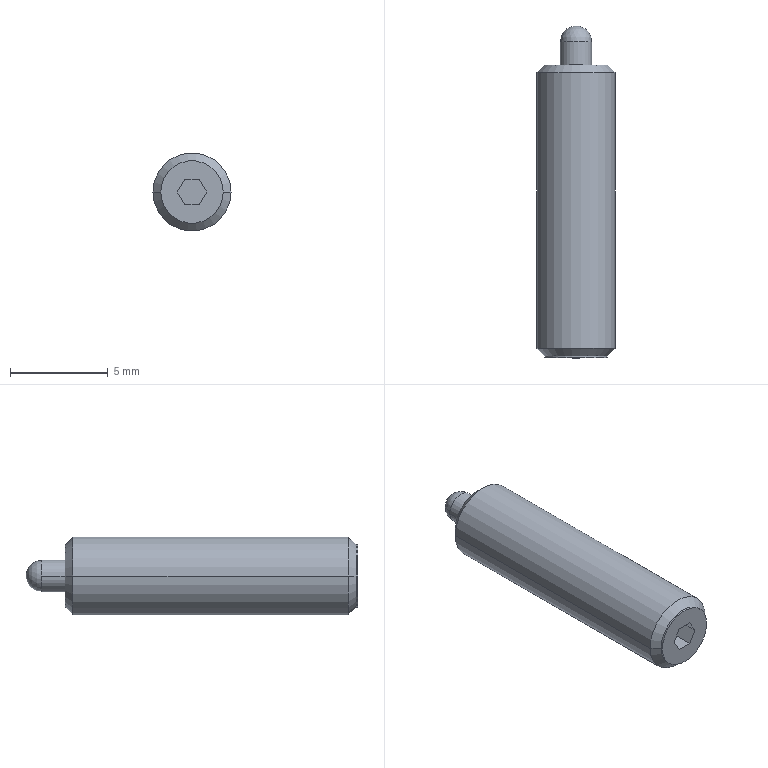Part | NX | 1 solid | 20 faces | box 4 x 17 x 4 mm | volume 187.749 mm3 | plane 9 | cylinder 6 | cone 4 | sphere 1 | commonest cylinder face diameters 1.6 x2 3.2 x2 4 x2
STEP:
#1=CARTESIAN_POINT('',(0.8,16.2,0.));
#2=VERTEX_POINT('',#1);
#3=CARTESIAN_POINT('',(-0.8,16.2,0.));
#4=VERTEX_POINT('',#3);
#5=CARTESIAN_POINT('',(0.,16.2,0.));
#6=DIRECTION('',(0.,1.,0.));
#7=DIRECTION('',(1.,0.,0.));
#8=AXIS2_PLACEMENT_3D('',#5,#6,#7);
#9=CIRCLE('',#8,0.8);
#10=EDGE_CURVE('',#2,#4,#9,.T.);
#11=ORIENTED_EDGE('',*,*,#10,.T.);
#12=CARTESIAN_POINT('',(0.,16.2,0.));
#13=DIRECTION('',(0.,1.,0.));
#14=DIRECTION('',(1.,0.,0.));
#15=AXIS2_PLACEMENT_3D('',#12,#13,#14);
#16=CIRCLE('',#15,0.8);
#17=EDGE_CURVE('',#4,#2,#16,.T.);
#18=ORIENTED_EDGE('',*,*,#17,.T.);
#19=EDGE_LOOP('',(#11,#18));
#20=FACE_BOUND('',#19,.T.);
#21=CARTESIAN_POINT('',(0.,16.2,0.));
#22=DIRECTION('',(0.,1.,0.));
#23=DIRECTION('',(1.,0.,0.));
#24=AXIS2_PLACEMENT_3D('',#21,#22,#23);
#25=SPHERICAL_SURFACE('',#24,0.8);
#26=ADVANCED_FACE('',(#20),#25,.T.);
#27=CARTESIAN_POINT('',(-0.7506,0.,0.));
#28=VERTEX_POINT('',#27);
#29=CARTESIAN_POINT('',(-0.3753,0.,-0.65));
#30=VERTEX_POINT('',#29);
#31=CARTESIAN_POINT('',(-0.7506,0.,0.));
#32=DIRECTION('',(0.5,0.,-0.866));
#33=VECTOR('',#32,1000.);
#34=LINE('',#31,#33);
#35=EDGE_CURVE('',#28,#30,#34,.T.);
#36=ORIENTED_EDGE('',*,*,#35,.T.);
#37=CARTESIAN_POINT('',(-0.3753,1.3,-0.65));
#38=VERTEX_POINT('',#37);
#39=CARTESIAN_POINT('',(-0.3753,1.3,-0.65));
#40=DIRECTION('',(0.,-1.,0.));
#41=VECTOR('',#40,1000.);
#42=LINE('',#39,#41);
#43=EDGE_CURVE('',#38,#30,#42,.T.);
#44=ORIENTED_EDGE('',*,*,#43,.F.);
#45=CARTESIAN_POINT('',(-0.7506,1.3,0.));
#46=VERTEX_POINT('',#45);
#47=CARTESIAN_POINT('',(-0.3753,1.3,-0.65));
#48=DIRECTION('',(-0.5,0.,0.866));
#49=VECTOR('',#48,1000.);
#50=LINE('',#47,#49);
#51=EDGE_CURVE('',#38,#46,#50,.T.);
#52=ORIENTED_EDGE('',*,*,#51,.T.);
#53=CARTESIAN_POINT('',(-0.7506,1.3,0.));
#54=DIRECTION('',(0.,-1.,0.));
#55=VECTOR('',#54,1000.);
#56=LINE('',#53,#55);
#57=EDGE_CURVE('',#46,#28,#56,.T.);
#58=ORIENTED_EDGE('',*,*,#57,.T.);
#59=EDGE_LOOP('',(#36,#44,#52,#58));
#60=FACE_BOUND('',#59,.T.);
#61=CARTESIAN_POINT('',(-0.7506,0.,0.));
#62=DIRECTION('',(-0.866,0.,-0.5));
#63=DIRECTION('',(-0.5,0.,0.866));
#64=AXIS2_PLACEMENT_3D('',#61,#62,#63);
#65=PLANE('',#64);
#66=ADVANCED_FACE('',(#60),#65,.F.);
#67=ORIENTED_EDGE('',*,*,#17,.F.);
#68=CARTESIAN_POINT('',(-0.8,15.,0.));
#69=VERTEX_POINT('',#68);
#70=CARTESIAN_POINT('',(-0.8,17.85,0.));
#71=DIRECTION('',(0.,-1.,0.));
#72=VECTOR('',#71,1000.);
#73=LINE('',#70,#72);
#74=EDGE_CURVE('',#69,#4,#73,.F.);
#75=ORIENTED_EDGE('',*,*,#74,.F.);
#76=CARTESIAN_POINT('',(0.8,15.,0.));
#77=VERTEX_POINT('',#76);
#78=CARTESIAN_POINT('',(0.,15.,0.));
#79=DIRECTION('',(0.,1.,0.));
#80=DIRECTION('',(1.,0.,0.));
#81=AXIS2_PLACEMENT_3D('',#78,#79,#80);
#82=CIRCLE('',#81,0.8);
#83=EDGE_CURVE('',#69,#77,#82,.T.);
#84=ORIENTED_EDGE('',*,*,#83,.T.);
#85=CARTESIAN_POINT('',(0.8,17.85,0.));
#86=DIRECTION('',(0.,-1.,0.));
#87=VECTOR('',#86,1000.);
#88=LINE('',#85,#87);
#89=EDGE_CURVE('',#77,#2,#88,.F.);
#90=ORIENTED_EDGE('',*,*,#89,.T.);
#91=EDGE_LOOP('',(#67,#75,#84,#90));
#92=FACE_BOUND('',#91,.T.);
#93=CARTESIAN_POINT('',(0.,17.85,0.));
#94=DIRECTION('',(0.,-1.,0.));
#95=DIRECTION('',(-1.,0.,0.));
#96=AXIS2_PLACEMENT_3D('',#93,#94,#95);
#97=CYLINDRICAL_SURFACE('',#96,0.8);
#98=ADVANCED_FACE('',(#92),#97,.T.);
#99=CARTESIAN_POINT('',(0.3753,0.,-0.65));
#100=VERTEX_POINT('',#99);
#101=CARTESIAN_POINT('',(0.3753,0.,-0.65));
#102=DIRECTION('',(-1.,0.,0.));
#103=VECTOR('',#102,1000.);
#104=LINE('',#101,#103);
#105=EDGE_CURVE('',#100,#30,#104,.T.);
#106=ORIENTED_EDGE('',*,*,#105,.F.);
#107=CARTESIAN_POINT('',(0.3753,1.3,-0.65));
#108=VERTEX_POINT('',#107);
#109=CARTESIAN_POINT('',(0.3753,1.3,-0.65));
#110=DIRECTION('',(0.,-1.,0.));
#111=VECTOR('',#110,1000.);
#112=LINE('',#109,#111);
#113=EDGE_CURVE('',#108,#100,#112,.T.);
#114=ORIENTED_EDGE('',*,*,#113,.F.);
#115=CARTESIAN_POINT('',(0.3753,1.3,-0.65));
#116=DIRECTION('',(-1.,0.,0.));
#117=VECTOR('',#116,1000.);
#118=LINE('',#115,#117);
#119=EDGE_CURVE('',#108,#38,#118,.T.);
#120=ORIENTED_EDGE('',*,*,#119,.T.);
#121=ORIENTED_EDGE('',*,*,#43,.T.);
#122=EDGE_LOOP('',(#106,#114,#120,#121));
#123=FACE_BOUND('',#122,.T.);
#124=CARTESIAN_POINT('',(-0.3753,0.,-0.65));
#125=DIRECTION('',(0.,0.,-1.));
#126=DIRECTION('',(0.,-1.,0.));
#127=AXIS2_PLACEMENT_3D('',#124,#125,#126);
#128=PLANE('',#127);
#129=ADVANCED_FACE('',(#123),#128,.F.);
#130=CARTESIAN_POINT('',(-1.6,15.,0.));
#131=VERTEX_POINT('',#130);
#132=CARTESIAN_POINT('',(1.6,15.,0.));
#133=VERTEX_POINT('',#132);
#134=CARTESIAN_POINT('',(0.,15.,0.));
#135=DIRECTION('',(0.,-1.,0.));
#136=DIRECTION('',(-1.,0.,0.));
#137=AXIS2_PLACEMENT_3D('',#134,#135,#136);
#138=CIRCLE('',#137,1.6);
#139=EDGE_CURVE('',#131,#133,#138,.T.);
#140=ORIENTED_EDGE('',*,*,#139,.F.);
#141=CARTESIAN_POINT('',(0.,15.,0.));
#142=DIRECTION('',(0.,-1.,0.));
#143=DIRECTION('',(-1.,0.,0.));
#144=AXIS2_PLACEMENT_3D('',#141,#142,#143);
#145=CIRCLE('',#144,1.6);
#146=EDGE_CURVE('',#133,#131,#145,.T.);
#147=ORIENTED_EDGE('',*,*,#146,.F.);
#148=EDGE_LOOP('',(#140,#147));
#149=FACE_BOUND('',#148,.T.);
#150=CARTESIAN_POINT('',(0.,15.,0.));
#151=DIRECTION('',(0.,1.,0.));
#152=DIRECTION('',(1.,0.,0.));
#153=AXIS2_PLACEMENT_3D('',#150,#151,#152);
#154=CIRCLE('',#153,0.8);
#155=EDGE_CURVE('',#77,#69,#154,.T.);
#156=ORIENTED_EDGE('',*,*,#155,.F.);
#157=ORIENTED_EDGE('',*,*,#83,.F.);
#158=EDGE_LOOP('',(#156,#157));
#159=FACE_BOUND('',#158,.T.);
#160=CARTESIAN_POINT('',(0.,15.,0.));
#161=DIRECTION('',(0.,-1.,0.));
#162=DIRECTION('',(0.,0.,-1.));
#163=AXIS2_PLACEMENT_3D('',#160,#161,#162);
#164=PLANE('',#163);
#165=ADVANCED_FACE('',(#149,#159),#164,.F.);
#166=ORIENTED_EDGE('',*,*,#139,.T.);
#167=CARTESIAN_POINT('',(2.,14.6,0.));
#168=VERTEX_POINT('',#167);
#169=CARTESIAN_POINT('',(1.8,14.8,0.));
#170=DIRECTION('',(0.7071,-0.7071,0.));
#171=VECTOR('',#170,1000.);
#172=LINE('',#169,#171);
#173=EDGE_CURVE('',#168,#133,#172,.F.);
#174=ORIENTED_EDGE('',*,*,#173,.F.);
#175=CARTESIAN_POINT('',(-2.,14.6,0.));
#176=VERTEX_POINT('',#175);
#177=CARTESIAN_POINT('',(0.,14.6,0.));
#178=DIRECTION('',(0.,-1.,0.));
#179=DIRECTION('',(-1.,0.,0.));
#180=AXIS2_PLACEMENT_3D('',#177,#178,#179);
#181=CIRCLE('',#180,2.);
#182=EDGE_CURVE('',#176,#168,#181,.T.);
#183=ORIENTED_EDGE('',*,*,#182,.F.);
#184=CARTESIAN_POINT('',(-1.8,14.8,0.));
#185=DIRECTION('',(-0.7071,-0.7071,0.));
#186=VECTOR('',#185,1000.);
#187=LINE('',#184,#186);
#188=EDGE_CURVE('',#176,#131,#187,.F.);
#189=ORIENTED_EDGE('',*,*,#188,.T.);
#190=EDGE_LOOP('',(#166,#174,#183,#189));
#191=FACE_BOUND('',#190,.T.);
#192=CARTESIAN_POINT('',(0.,14.8,0.));
#193=DIRECTION('',(0.,-1.,0.));
#194=DIRECTION('',(-1.,0.,0.));
#195=AXIS2_PLACEMENT_3D('',#192,#193,#194);
#196=CONICAL_SURFACE('',#195,1.8,0.7854);
#197=ADVANCED_FACE('',(#191),#196,.T.);
#198=CARTESIAN_POINT('',(0.3753,1.3,0.65));
#199=VERTEX_POINT('',#198);
#200=CARTESIAN_POINT('',(0.7506,1.3,0.));
#201=VERTEX_POINT('',#200);
#202=CARTESIAN_POINT('',(0.3753,1.3,0.65));
#203=DIRECTION('',(0.5,0.,-0.866));
#204=VECTOR('',#203,1000.);
#205=LINE('',#202,#204);
#206=EDGE_CURVE('',#199,#201,#205,.T.);
#207=ORIENTED_EDGE('',*,*,#206,.F.);
#208=CARTESIAN_POINT('',(-0.3753,1.3,0.65));
#209=VERTEX_POINT('',#208);
#210=CARTESIAN_POINT('',(-0.3753,1.3,0.65));
#211=DIRECTION('',(1.,0.,0.));
#212=VECTOR('',#211,1000.);
#213=LINE('',#210,#212);
#214=EDGE_CURVE('',#209,#199,#213,.T.);
#215=ORIENTED_EDGE('',*,*,#214,.F.);
#216=CARTESIAN_POINT('',(-0.7506,1.3,0.));
#217=DIRECTION('',(0.5,0.,0.866));
#218=VECTOR('',#217,1000.);
#219=LINE('',#216,#218);
#220=EDGE_CURVE('',#46,#209,#219,.T.);
#221=ORIENTED_EDGE('',*,*,#220,.F.);
#222=ORIENTED_EDGE('',*,*,#51,.F.);
#223=ORIENTED_EDGE('',*,*,#119,.F.);
#224=CARTESIAN_POINT('',(0.7506,1.3,0.));
#225=DIRECTION('',(-0.5,0.,-0.866));
#226=VECTOR('',#225,1000.);
#227=LINE('',#224,#226);
#228=EDGE_CURVE('',#201,#108,#227,.T.);
#229=ORIENTED_EDGE('',*,*,#228,.F.);
#230=EDGE_LOOP('',(#207,#215,#221,#222,#223,#229));
#231=FACE_BOUND('',#230,.T.);
#232=CARTESIAN_POINT('',(0.,1.3,0.));
#233=DIRECTION('',(0.,-1.,0.));
#234=DIRECTION('',(0.,0.,-1.));
#235=AXIS2_PLACEMENT_3D('',#232,#233,#234);
#236=PLANE('',#235);
#237=ADVANCED_FACE('',(#231),#236,.T.);
#238=ORIENTED_EDGE('',*,*,#182,.T.);
#239=CARTESIAN_POINT('',(2.,0.5,0.));
#240=VERTEX_POINT('',#239);
#241=CARTESIAN_POINT('',(2.,17.85,0.));
#242=DIRECTION('',(0.,-1.,0.));
#243=VECTOR('',#242,1000.);
#244=LINE('',#241,#243);
#245=EDGE_CURVE('',#168,#240,#244,.T.);
#246=ORIENTED_EDGE('',*,*,#245,.T.);
#247=CARTESIAN_POINT('',(-2.,0.5,0.));
#248=VERTEX_POINT('',#247);
#249=CARTESIAN_POINT('',(0.,0.5,0.));
#250=DIRECTION('',(0.,1.,0.));
#251=DIRECTION('',(1.,0.,0.));
#252=AXIS2_PLACEMENT_3D('',#249,#250,#251);
#253=CIRCLE('',#252,2.);
#254=EDGE_CURVE('',#240,#248,#253,.T.);
#255=ORIENTED_EDGE('',*,*,#254,.T.);
#256=CARTESIAN_POINT('',(-2.,17.85,0.));
#257=DIRECTION('',(0.,-1.,0.));
#258=VECTOR('',#257,1000.);
#259=LINE('',#256,#258);
#260=EDGE_CURVE('',#176,#248,#259,.T.);
#261=ORIENTED_EDGE('',*,*,#260,.F.);
#262=EDGE_LOOP('',(#238,#246,#255,#261));
#263=FACE_BOUND('',#262,.T.);
#264=CARTESIAN_POINT('',(0.,17.85,0.));
#265=DIRECTION('',(0.,-1.,0.));
#266=DIRECTION('',(-1.,0.,0.));
#267=AXIS2_PLACEMENT_3D('',#264,#265,#266);
#268=CYLINDRICAL_SURFACE('',#267,2.);
#269=ADVANCED_FACE('',(#263),#268,.T.);
#270=CARTESIAN_POINT('',(-0.3753,0.,0.65));
#271=VERTEX_POINT('',#270);
#272=CARTESIAN_POINT('',(-0.3753,0.,0.65));
#273=DIRECTION('',(-0.5,0.,-0.866));
#274=VECTOR('',#273,1000.);
#275=LINE('',#272,#274);
#276=EDGE_CURVE('',#271,#28,#275,.T.);
#277=ORIENTED_EDGE('',*,*,#276,.T.);
#278=ORIENTED_EDGE('',*,*,#57,.F.);
#279=ORIENTED_EDGE('',*,*,#220,.T.);
#280=CARTESIAN_POINT('',(-0.3753,1.3,0.65));
#281=DIRECTION('',(0.,-1.,0.));
#282=VECTOR('',#281,1000.);
#283=LINE('',#280,#282);
#284=EDGE_CURVE('',#209,#271,#283,.T.);
#285=ORIENTED_EDGE('',*,*,#284,.T.);
#286=EDGE_LOOP('',(#277,#278,#279,#285));
#287=FACE_BOUND('',#286,.T.);
#288=CARTESIAN_POINT('',(-0.3753,0.,0.65));
#289=DIRECTION('',(-0.866,0.,0.5));
#290=DIRECTION('',(0.,1.,0.));
#291=AXIS2_PLACEMENT_3D('',#288,#289,#290);
#292=PLANE('',#291);
#293=ADVANCED_FACE('',(#287),#292,.F.);
#294=CARTESIAN_POINT('',(-1.6,0.1,0.));
#295=VERTEX_POINT('',#294);
#296=CARTESIAN_POINT('',(1.6,0.1,0.));
#297=VERTEX_POINT('',#296);
#298=CARTESIAN_POINT('',(0.,0.1,0.));
#299=DIRECTION('',(0.,-1.,0.));
#300=DIRECTION('',(-1.,0.,0.));
#301=AXIS2_PLACEMENT_3D('',#298,#299,#300);
#302=CIRCLE('',#301,1.6);
#303=EDGE_CURVE('',#295,#297,#302,.T.);
#304=ORIENTED_EDGE('',*,*,#303,.F.);
#305=CARTESIAN_POINT('',(-1.8,0.3,0.));
#306=DIRECTION('',(-0.7071,0.7071,0.));
#307=VECTOR('',#306,1000.);
#308=LINE('',#305,#307);
#309=EDGE_CURVE('',#248,#295,#308,.F.);
#310=ORIENTED_EDGE('',*,*,#309,.F.);
#311=ORIENTED_EDGE('',*,*,#254,.F.);
#312=CARTESIAN_POINT('',(1.8,0.3,0.));
#313=DIRECTION('',(0.7071,0.7071,0.));
#314=VECTOR('',#313,1000.);
#315=LINE('',#312,#314);
#316=EDGE_CURVE('',#240,#297,#315,.F.);
#317=ORIENTED_EDGE('',*,*,#316,.T.);
#318=EDGE_LOOP('',(#304,#310,#311,#317));
#319=FACE_BOUND('',#318,.T.);
#320=CARTESIAN_POINT('',(0.,0.3,0.));
#321=DIRECTION('',(0.,1.,0.));
#322=DIRECTION('',(1.,0.,0.));
#323=AXIS2_PLACEMENT_3D('',#320,#321,#322);
#324=CONICAL_SURFACE('',#323,1.8,0.7854);
#325=ADVANCED_FACE('',(#319),#324,.T.);
#326=CARTESIAN_POINT('',(0.7506,0.,0.));
#327=VERTEX_POINT('',#326);
#328=CARTESIAN_POINT('',(0.3753,0.,-0.65));
#329=DIRECTION('',(0.5,0.,0.866));
#330=VECTOR('',#329,1000.);
#331=LINE('',#328,#330);
#332=EDGE_CURVE('',#100,#327,#331,.T.);
#333=ORIENTED_EDGE('',*,*,#332,.T.);
#334=CARTESIAN_POINT('',(0.7506,1.3,0.));
#335=DIRECTION('',(0.,-1.,0.));
#336=VECTOR('',#335,1000.);
#337=LINE('',#334,#336);
#338=EDGE_CURVE('',#201,#327,#337,.T.);
#339=ORIENTED_EDGE('',*,*,#338,.F.);
#340=ORIENTED_EDGE('',*,*,#228,.T.);
#341=ORIENTED_EDGE('',*,*,#113,.T.);
#342=EDGE_LOOP('',(#333,#339,#340,#341));
#343=FACE_BOUND('',#342,.T.);
#344=CARTESIAN_POINT('',(0.3753,0.,-0.65));
#345=DIRECTION('',(0.866,0.,-0.5));
#346=DIRECTION('',(0.,-1.,0.));
#347=AXIS2_PLACEMENT_3D('',#344,#345,#346);
#348=PLANE('',#347);
#349=ADVANCED_FACE('',(#343),#348,.F.);
#350=CARTESIAN_POINT('',(-1.6,0.,0.));
#351=VERTEX_POINT('',#350);
#352=CARTESIAN_POINT('',(1.6,0.,0.));
#353=VERTEX_POINT('',#352);
#354=CARTESIAN_POINT('',(0.,0.,0.));
#355=DIRECTION('',(0.,1.,0.));
#356=DIRECTION('',(1.,0.,0.));
#357=AXIS2_PLACEMENT_3D('',#354,#355,#356);
#358=CIRCLE('',#357,1.6);
#359=EDGE_CURVE('',#351,#353,#358,.T.);
#360=ORIENTED_EDGE('',*,*,#359,.T.);
#361=CARTESIAN_POINT('',(1.6,17.85,0.));
#362=DIRECTION('',(0.,-1.,0.));
#363=VECTOR('',#362,1000.);
#364=LINE('',#361,#363);
#365=EDGE_CURVE('',#297,#353,#364,.T.);
#366=ORIENTED_EDGE('',*,*,#365,.F.);
#367=CARTESIAN_POINT('',(0.,0.1,0.));
#368=DIRECTION('',(0.,-1.,0.));
#369=DIRECTION('',(-1.,0.,0.));
#370=AXIS2_PLACEMENT_3D('',#367,#368,#369);
#371=CIRCLE('',#370,1.6);
#372=EDGE_CURVE('',#297,#295,#371,.T.);
#373=ORIENTED_EDGE('',*,*,#372,.T.);
#374=CARTESIAN_POINT('',(-1.6,17.85,0.));
#375=DIRECTION('',(0.,-1.,0.));
#376=VECTOR('',#375,1000.);
#377=LINE('',#374,#376);
#378=EDGE_CURVE('',#295,#351,#377,.T.);
#379=ORIENTED_EDGE('',*,*,#378,.T.);
#380=EDGE_LOOP('',(#360,#366,#373,#379));
#381=FACE_BOUND('',#380,.T.);
#382=CARTESIAN_POINT('',(0.,17.85,0.));
#383=DIRECTION('',(0.,-1.,0.));
#384=DIRECTION('',(-1.,0.,0.));
#385=AXIS2_PLACEMENT_3D('',#382,#383,#384);
#386=CYLINDRICAL_SURFACE('',#385,1.6);
#387=ADVANCED_FACE('',(#381),#386,.T.);
#388=CARTESIAN_POINT('',(0.3753,0.,0.65));
#389=VERTEX_POINT('',#388);
#390=CARTESIAN_POINT('',(-0.3753,0.,0.65));
#391=DIRECTION('',(1.,0.,0.));
#392=VECTOR('',#391,1000.);
#393=LINE('',#390,#392);
#394=EDGE_CURVE('',#271,#389,#393,.T.);
#395=ORIENTED_EDGE('',*,*,#394,.F.);
#396=ORIENTED_EDGE('',*,*,#284,.F.);
#397=ORIENTED_EDGE('',*,*,#214,.T.);
#398=CARTESIAN_POINT('',(0.3753,1.3,0.65));
#399=DIRECTION('',(0.,-1.,0.));
#400=VECTOR('',#399,1000.);
#401=LINE('',#398,#400);
#402=EDGE_CURVE('',#199,#389,#401,.T.);
#403=ORIENTED_EDGE('',*,*,#402,.T.);
#404=EDGE_LOOP('',(#395,#396,#397,#403));
#405=FACE_BOUND('',#404,.T.);
#406=CARTESIAN_POINT('',(0.3753,0.,0.65));
#407=DIRECTION('',(0.,0.,1.));
#408=DIRECTION('',(1.,0.,0.));
#409=AXIS2_PLACEMENT_3D('',#406,#407,#408);
#410=PLANE('',#409);
#411=ADVANCED_FACE('',(#405),#410,.F.);
#412=ORIENTED_EDGE('',*,*,#359,.F.);
#413=CARTESIAN_POINT('',(0.,0.,0.));
#414=DIRECTION('',(0.,1.,0.));
#415=DIRECTION('',(1.,0.,0.));
#416=AXIS2_PLACEMENT_3D('',#413,#414,#415);
#417=CIRCLE('',#416,1.6);
#418=EDGE_CURVE('',#353,#351,#417,.T.);
#419=ORIENTED_EDGE('',*,*,#418,.F.);
#420=EDGE_LOOP('',(#412,#419));
#421=FACE_BOUND('',#420,.T.);
#422=CARTESIAN_POINT('',(0.7506,0.,0.));
#423=DIRECTION('',(-0.5,0.,0.866));
#424=VECTOR('',#423,1000.);
#425=LINE('',#422,#424);
#426=EDGE_CURVE('',#327,#389,#425,.T.);
#427=ORIENTED_EDGE('',*,*,#426,.F.);
#428=ORIENTED_EDGE('',*,*,#332,.F.);
#429=ORIENTED_EDGE('',*,*,#105,.T.);
#430=ORIENTED_EDGE('',*,*,#35,.F.);
#431=ORIENTED_EDGE('',*,*,#276,.F.);
#432=ORIENTED_EDGE('',*,*,#394,.T.);
#433=EDGE_LOOP('',(#427,#428,#429,#430,#431,#432));
#434=FACE_BOUND('',#433,.T.);
#435=CARTESIAN_POINT('',(0.,0.,0.));
#436=DIRECTION('',(0.,-1.,0.));
#437=DIRECTION('',(0.,0.,-1.));
#438=AXIS2_PLACEMENT_3D('',#435,#436,#437);
#439=PLANE('',#438);
#440=ADVANCED_FACE('',(#421,#434),#439,.T.);
#441=ORIENTED_EDGE('',*,*,#426,.T.);
#442=ORIENTED_EDGE('',*,*,#402,.F.);
#443=ORIENTED_EDGE('',*,*,#206,.T.);
#444=ORIENTED_EDGE('',*,*,#338,.T.);
#445=EDGE_LOOP('',(#441,#442,#443,#444));
#446=FACE_BOUND('',#445,.T.);
#447=CARTESIAN_POINT('',(0.7506,0.,0.));
#448=DIRECTION('',(0.866,0.,0.5));
#449=DIRECTION('',(0.,-1.,0.));
#450=AXIS2_PLACEMENT_3D('',#447,#448,#449);
#451=PLANE('',#450);
#452=ADVANCED_FACE('',(#446),#451,.F.);
#453=ORIENTED_EDGE('',*,*,#303,.T.);
#454=ORIENTED_EDGE('',*,*,#365,.T.);
#455=ORIENTED_EDGE('',*,*,#418,.T.);
#456=ORIENTED_EDGE('',*,*,#378,.F.);
#457=EDGE_LOOP('',(#453,#454,#455,#456));
#458=FACE_BOUND('',#457,.T.);
#459=CARTESIAN_POINT('',(0.,17.85,0.));
#460=DIRECTION('',(0.,-1.,0.));
#461=DIRECTION('',(-1.,0.,0.));
#462=AXIS2_PLACEMENT_3D('',#459,#460,#461);
#463=CYLINDRICAL_SURFACE('',#462,1.6);
#464=ADVANCED_FACE('',(#458),#463,.T.);
#465=CARTESIAN_POINT('',(0.,0.5,0.));
#466=DIRECTION('',(0.,1.,0.));
#467=DIRECTION('',(1.,0.,0.));
#468=AXIS2_PLACEMENT_3D('',#465,#466,#467);
#469=CIRCLE('',#468,2.);
#470=EDGE_CURVE('',#248,#240,#469,.T.);
#471=ORIENTED_EDGE('',*,*,#470,.F.);
#472=ORIENTED_EDGE('',*,*,#309,.T.);
#473=ORIENTED_EDGE('',*,*,#372,.F.);
#474=ORIENTED_EDGE('',*,*,#316,.F.);
#475=EDGE_LOOP('',(#471,#472,#473,#474));
#476=FACE_BOUND('',#475,.T.);
#477=CARTESIAN_POINT('',(0.,0.3,0.));
#478=DIRECTION('',(0.,1.,0.));
#479=DIRECTION('',(1.,0.,0.));
#480=AXIS2_PLACEMENT_3D('',#477,#478,#479);
#481=CONICAL_SURFACE('',#480,1.8,0.7854);
#482=ADVANCED_FACE('',(#476),#481,.T.);
#483=ORIENTED_EDGE('',*,*,#470,.T.);
#484=ORIENTED_EDGE('',*,*,#245,.F.);
#485=CARTESIAN_POINT('',(0.,14.6,0.));
#486=DIRECTION('',(0.,-1.,0.));
#487=DIRECTION('',(-1.,0.,0.));
#488=AXIS2_PLACEMENT_3D('',#485,#486,#487);
#489=CIRCLE('',#488,2.);
#490=EDGE_CURVE('',#168,#176,#489,.T.);
#491=ORIENTED_EDGE('',*,*,#490,.T.);
#492=ORIENTED_EDGE('',*,*,#260,.T.);
#493=EDGE_LOOP('',(#483,#484,#491,#492));
#494=FACE_BOUND('',#493,.T.);
#495=CARTESIAN_POINT('',(0.,17.85,0.));
#496=DIRECTION('',(0.,-1.,0.));
#497=DIRECTION('',(-1.,0.,0.));
#498=AXIS2_PLACEMENT_3D('',#495,#496,#497);
#499=CYLINDRICAL_SURFACE('',#498,2.);
#500=ADVANCED_FACE('',(#494),#499,.T.);
#501=ORIENTED_EDGE('',*,*,#188,.F.);
#502=ORIENTED_EDGE('',*,*,#490,.F.);
#503=ORIENTED_EDGE('',*,*,#173,.T.);
#504=ORIENTED_EDGE('',*,*,#146,.T.);
#505=EDGE_LOOP('',(#501,#502,#503,#504));
#506=FACE_BOUND('',#505,.T.);
#507=CARTESIAN_POINT('',(0.,14.8,0.));
#508=DIRECTION('',(0.,-1.,0.));
#509=DIRECTION('',(-1.,0.,0.));
#510=AXIS2_PLACEMENT_3D('',#507,#508,#509);
#511=CONICAL_SURFACE('',#510,1.8,0.7854);
#512=ADVANCED_FACE('',(#506),#511,.T.);
#513=ORIENTED_EDGE('',*,*,#155,.T.);
#514=ORIENTED_EDGE('',*,*,#74,.T.);
#515=ORIENTED_EDGE('',*,*,#10,.F.);
#516=ORIENTED_EDGE('',*,*,#89,.F.);
#517=EDGE_LOOP('',(#513,#514,#515,#516));
#518=FACE_BOUND('',#517,.T.);
#519=CARTESIAN_POINT('',(0.,17.85,0.));
#520=DIRECTION('',(0.,-1.,0.));
#521=DIRECTION('',(-1.,0.,0.));
#522=AXIS2_PLACEMENT_3D('',#519,#520,#521);
#523=CYLINDRICAL_SURFACE('',#522,0.8);
#524=ADVANCED_FACE('',(#518),#523,.T.);
#525=CLOSED_SHELL('',(#26,#66,#98,#129,#165,#197,#237,#269,#293,#325,#349,#387,#411,#440,#452,#464,#482,#500,#512,#524));
#526=MANIFOLD_SOLID_BREP('',#525);
#527=(LENGTH_UNIT()NAMED_UNIT(*)SI_UNIT(.MILLI.,.METRE.));
#528=UNCERTAINTY_MEASURE_WITH_UNIT(LENGTH_MEASURE(0.00001),#527,'','');
#529=(NAMED_UNIT(*)PLANE_ANGLE_UNIT()SI_UNIT($,.RADIAN.));
#530=(NAMED_UNIT(*)SI_UNIT($,.STERADIAN.)SOLID_ANGLE_UNIT());
#531=(GEOMETRIC_REPRESENTATION_CONTEXT(3)GLOBAL_UNCERTAINTY_ASSIGNED_CONTEXT((#528))GLOBAL_UNIT_ASSIGNED_CONTEXT((#527,#529,#530))REPRESENTATION_CONTEXT('',''));
#532=ADVANCED_BREP_SHAPE_REPRESENTATION('',(#526),#531);